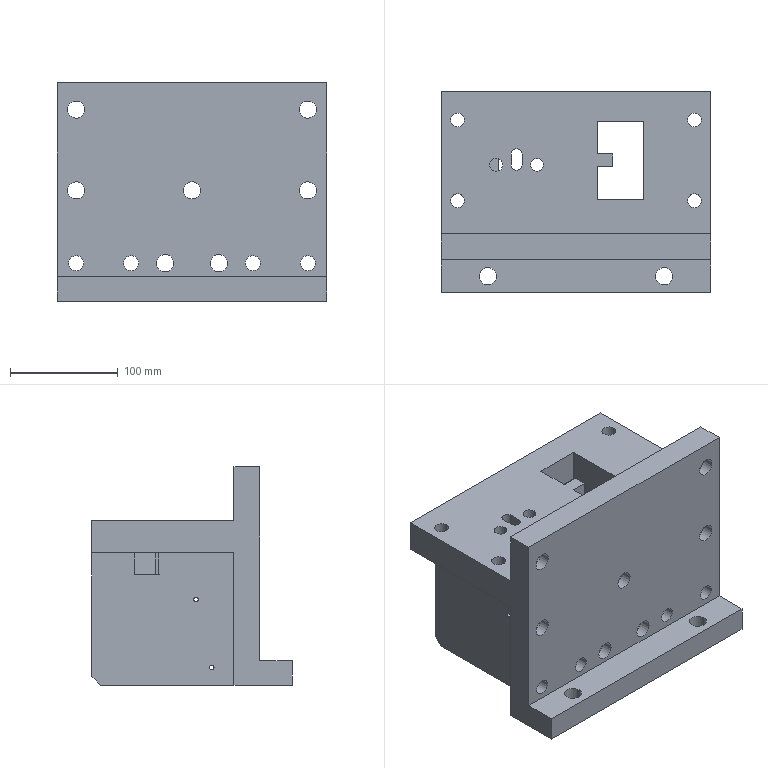Part | STEP file | GA KHUON COI KHONG LOGO | 1 solid | 103 faces | box 250 x 186 x 203 mm | volume 2822642 mm3 | cylinder 62 | plane 41 | commonest cylinder face diameters 16 x18 23 x14 13 x8 14 x8 4.134 x4 4.343 x4